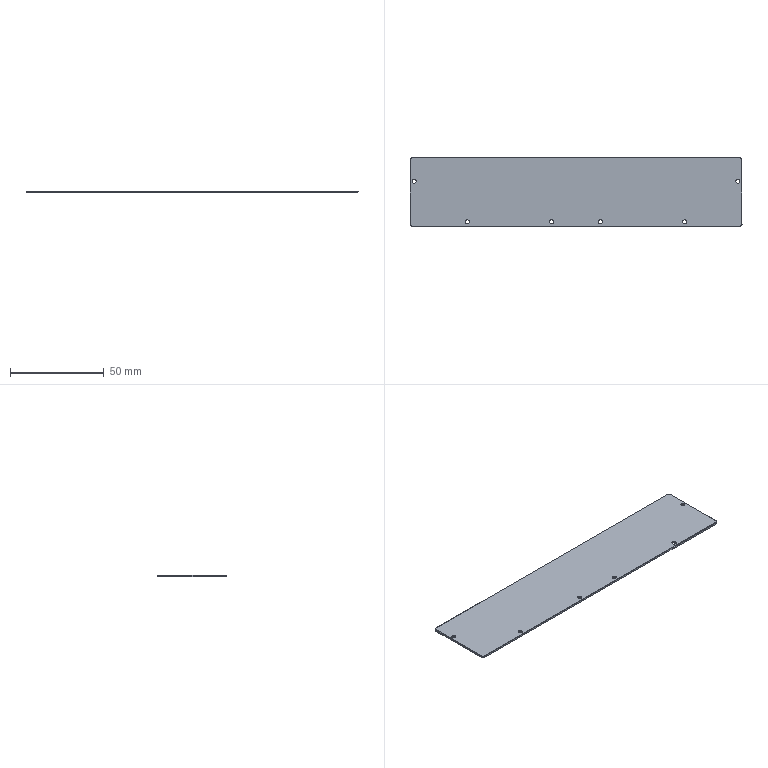Part | SolidWorks | features BaseBody 1 | 1 solid | 42 faces | box 177 x 36.8 x 1 mm | volume 6475 mm3 | cone 16 | cylinder 16 | plane 10 | commonest cylinder face diameters 2.2 x12 2.6 x4
STEP:
#1=CARTESIAN_POINT('',(-59.1,-64.9,0.5));
#2=VERTEX_POINT('',#1);
#3=CARTESIAN_POINT('',(-56.9,-64.9,0.5));
#4=VERTEX_POINT('',#3);
#5=CARTESIAN_POINT('',(-58.,-64.9,0.5));
#6=DIRECTION('',(0.,0.,1.));
#7=DIRECTION('',(0.,-1.,0.));
#8=AXIS2_PLACEMENT_3D('',#5,#6,#7);
#9=CIRCLE('',#8,1.1);
#10=EDGE_CURVE('',#2,#4,#9,.T.);
#11=ORIENTED_EDGE('',*,*,#10,.T.);
#12=CARTESIAN_POINT('',(-56.4,-64.9,0.000000001));
#13=VERTEX_POINT('',#12);
#14=CARTESIAN_POINT('',(-56.9,-64.9,0.5));
#15=DIRECTION('',(0.7071,0.,-0.7071));
#16=VECTOR('',#15,1000.);
#17=LINE('',#14,#16);
#18=EDGE_CURVE('',#4,#13,#17,.T.);
#19=ORIENTED_EDGE('',*,*,#18,.T.);
#20=CARTESIAN_POINT('',(-59.6,-64.9,0.000000001));
#21=VERTEX_POINT('',#20);
#22=CARTESIAN_POINT('',(-58.,-64.9,0.000000001));
#23=DIRECTION('',(0.,0.,-1.));
#24=DIRECTION('',(-1.,0.,0.));
#25=AXIS2_PLACEMENT_3D('',#22,#23,#24);
#26=CIRCLE('',#25,1.6);
#27=EDGE_CURVE('',#13,#21,#26,.T.);
#28=ORIENTED_EDGE('',*,*,#27,.T.);
#29=CARTESIAN_POINT('',(-59.1,-64.9,0.5));
#30=DIRECTION('',(-0.7071,0.,-0.7071));
#31=VECTOR('',#30,1000.);
#32=LINE('',#29,#31);
#33=EDGE_CURVE('',#2,#21,#32,.T.);
#34=ORIENTED_EDGE('',*,*,#33,.F.);
#35=EDGE_LOOP('',(#11,#19,#28,#34));
#36=FACE_OUTER_BOUND('',#35,.T.);
#37=CARTESIAN_POINT('',(-58.,-64.9,0.5));
#38=DIRECTION('',(0.,0.,-1.));
#39=DIRECTION('',(-1.,0.,0.));
#40=AXIS2_PLACEMENT_3D('',#37,#38,#39);
#41=CONICAL_SURFACE('',#40,1.1,0.7854);
#42=ADVANCED_FACE('',(#36),#41,.F.);
#43=CARTESIAN_POINT('',(56.9,-64.9,0.5));
#44=VERTEX_POINT('',#43);
#45=CARTESIAN_POINT('',(59.1,-64.9,0.5));
#46=VERTEX_POINT('',#45);
#47=CARTESIAN_POINT('',(58.,-64.9,0.5));
#48=DIRECTION('',(0.,0.,1.));
#49=DIRECTION('',(0.,-1.,0.));
#50=AXIS2_PLACEMENT_3D('',#47,#48,#49);
#51=CIRCLE('',#50,1.1);
#52=EDGE_CURVE('',#44,#46,#51,.T.);
#53=ORIENTED_EDGE('',*,*,#52,.T.);
#54=CARTESIAN_POINT('',(59.6,-64.9,0.000000001));
#55=VERTEX_POINT('',#54);
#56=CARTESIAN_POINT('',(59.1,-64.9,0.5));
#57=DIRECTION('',(0.7071,0.,-0.7071));
#58=VECTOR('',#57,1000.);
#59=LINE('',#56,#58);
#60=EDGE_CURVE('',#46,#55,#59,.T.);
#61=ORIENTED_EDGE('',*,*,#60,.T.);
#62=CARTESIAN_POINT('',(56.4,-64.9,0.000000001));
#63=VERTEX_POINT('',#62);
#64=CARTESIAN_POINT('',(58.,-64.9,0.000000001));
#65=DIRECTION('',(0.,0.,-1.));
#66=DIRECTION('',(-1.,0.,0.));
#67=AXIS2_PLACEMENT_3D('',#64,#65,#66);
#68=CIRCLE('',#67,1.6);
#69=EDGE_CURVE('',#55,#63,#68,.T.);
#70=ORIENTED_EDGE('',*,*,#69,.T.);
#71=CARTESIAN_POINT('',(56.9,-64.9,0.5));
#72=DIRECTION('',(-0.7071,0.,-0.7071));
#73=VECTOR('',#72,1000.);
#74=LINE('',#71,#73);
#75=EDGE_CURVE('',#44,#63,#74,.T.);
#76=ORIENTED_EDGE('',*,*,#75,.F.);
#77=EDGE_LOOP('',(#53,#61,#70,#76));
#78=FACE_OUTER_BOUND('',#77,.T.);
#79=CARTESIAN_POINT('',(58.,-64.9,0.5));
#80=DIRECTION('',(0.,0.,-1.));
#81=DIRECTION('',(-1.,0.,0.));
#82=AXIS2_PLACEMENT_3D('',#79,#80,#81);
#83=CONICAL_SURFACE('',#82,1.1,0.7854);
#84=ADVANCED_FACE('',(#78),#83,.F.);
#85=CARTESIAN_POINT('',(-87.4,-43.2,0.5));
#86=VERTEX_POINT('',#85);
#87=CARTESIAN_POINT('',(-85.2,-43.2,0.5));
#88=VERTEX_POINT('',#87);
#89=CARTESIAN_POINT('',(-86.3,-43.2,0.5));
#90=DIRECTION('',(0.,0.,1.));
#91=DIRECTION('',(0.,-1.,0.));
#92=AXIS2_PLACEMENT_3D('',#89,#90,#91);
#93=CIRCLE('',#92,1.1);
#94=EDGE_CURVE('',#86,#88,#93,.T.);
#95=ORIENTED_EDGE('',*,*,#94,.T.);
#96=CARTESIAN_POINT('',(-84.7,-43.2,0.000000001));
#97=VERTEX_POINT('',#96);
#98=CARTESIAN_POINT('',(-85.2,-43.2,0.5));
#99=DIRECTION('',(0.7071,0.,-0.7071));
#100=VECTOR('',#99,1000.);
#101=LINE('',#98,#100);
#102=EDGE_CURVE('',#88,#97,#101,.T.);
#103=ORIENTED_EDGE('',*,*,#102,.T.);
#104=CARTESIAN_POINT('',(-87.9,-43.2,0.000000001));
#105=VERTEX_POINT('',#104);
#106=CARTESIAN_POINT('',(-86.3,-43.2,0.000000001));
#107=DIRECTION('',(0.,0.,-1.));
#108=DIRECTION('',(-1.,0.,0.));
#109=AXIS2_PLACEMENT_3D('',#106,#107,#108);
#110=CIRCLE('',#109,1.6);
#111=EDGE_CURVE('',#97,#105,#110,.T.);
#112=ORIENTED_EDGE('',*,*,#111,.T.);
#113=CARTESIAN_POINT('',(-87.4,-43.2,0.5));
#114=DIRECTION('',(-0.7071,0.,-0.7071));
#115=VECTOR('',#114,1000.);
#116=LINE('',#113,#115);
#117=EDGE_CURVE('',#86,#105,#116,.T.);
#118=ORIENTED_EDGE('',*,*,#117,.F.);
#119=EDGE_LOOP('',(#95,#103,#112,#118));
#120=FACE_OUTER_BOUND('',#119,.T.);
#121=CARTESIAN_POINT('',(-86.3,-43.2,0.5));
#122=DIRECTION('',(0.,0.,-1.));
#123=DIRECTION('',(-1.,0.,0.));
#124=AXIS2_PLACEMENT_3D('',#121,#122,#123);
#125=CONICAL_SURFACE('',#124,1.1,0.7854);
#126=ADVANCED_FACE('',(#120),#125,.F.);
#127=CARTESIAN_POINT('',(-14.1,-64.9,0.5));
#128=VERTEX_POINT('',#127);
#129=CARTESIAN_POINT('',(-11.9,-64.9,0.5));
#130=VERTEX_POINT('',#129);
#131=CARTESIAN_POINT('',(-13.,-64.9,0.5));
#132=DIRECTION('',(0.,0.,1.));
#133=DIRECTION('',(0.,-1.,0.));
#134=AXIS2_PLACEMENT_3D('',#131,#132,#133);
#135=CIRCLE('',#134,1.1);
#136=EDGE_CURVE('',#128,#130,#135,.T.);
#137=ORIENTED_EDGE('',*,*,#136,.T.);
#138=CARTESIAN_POINT('',(-11.4,-64.9,0.000000001));
#139=VERTEX_POINT('',#138);
#140=CARTESIAN_POINT('',(-11.9,-64.9,0.5));
#141=DIRECTION('',(0.7071,0.,-0.7071));
#142=VECTOR('',#141,1000.);
#143=LINE('',#140,#142);
#144=EDGE_CURVE('',#130,#139,#143,.T.);
#145=ORIENTED_EDGE('',*,*,#144,.T.);
#146=CARTESIAN_POINT('',(-14.6,-64.9,0.000000001));
#147=VERTEX_POINT('',#146);
#148=CARTESIAN_POINT('',(-13.,-64.9,0.000000001));
#149=DIRECTION('',(0.,0.,-1.));
#150=DIRECTION('',(-1.,0.,0.));
#151=AXIS2_PLACEMENT_3D('',#148,#149,#150);
#152=CIRCLE('',#151,1.6);
#153=EDGE_CURVE('',#139,#147,#152,.T.);
#154=ORIENTED_EDGE('',*,*,#153,.T.);
#155=CARTESIAN_POINT('',(-14.1,-64.9,0.5));
#156=DIRECTION('',(-0.7071,0.,-0.7071));
#157=VECTOR('',#156,1000.);
#158=LINE('',#155,#157);
#159=EDGE_CURVE('',#128,#147,#158,.T.);
#160=ORIENTED_EDGE('',*,*,#159,.F.);
#161=EDGE_LOOP('',(#137,#145,#154,#160));
#162=FACE_OUTER_BOUND('',#161,.T.);
#163=CARTESIAN_POINT('',(-13.,-64.9,0.5));
#164=DIRECTION('',(0.,0.,-1.));
#165=DIRECTION('',(-1.,0.,0.));
#166=AXIS2_PLACEMENT_3D('',#163,#164,#165);
#167=CONICAL_SURFACE('',#166,1.1,0.7854);
#168=ADVANCED_FACE('',(#162),#167,.F.);
#169=CARTESIAN_POINT('',(11.9,-64.9,0.5));
#170=VERTEX_POINT('',#169);
#171=CARTESIAN_POINT('',(14.1,-64.9,0.5));
#172=VERTEX_POINT('',#171);
#173=CARTESIAN_POINT('',(13.,-64.9,0.5));
#174=DIRECTION('',(0.,0.,1.));
#175=DIRECTION('',(0.,-1.,0.));
#176=AXIS2_PLACEMENT_3D('',#173,#174,#175);
#177=CIRCLE('',#176,1.1);
#178=EDGE_CURVE('',#170,#172,#177,.T.);
#179=ORIENTED_EDGE('',*,*,#178,.T.);
#180=CARTESIAN_POINT('',(14.6,-64.9,0.000000001));
#181=VERTEX_POINT('',#180);
#182=CARTESIAN_POINT('',(14.1,-64.9,0.5));
#183=DIRECTION('',(0.7071,0.,-0.7071));
#184=VECTOR('',#183,1000.);
#185=LINE('',#182,#184);
#186=EDGE_CURVE('',#172,#181,#185,.T.);
#187=ORIENTED_EDGE('',*,*,#186,.T.);
#188=CARTESIAN_POINT('',(11.4,-64.9,0.000000001));
#189=VERTEX_POINT('',#188);
#190=CARTESIAN_POINT('',(13.,-64.9,0.000000001));
#191=DIRECTION('',(0.,0.,-1.));
#192=DIRECTION('',(-1.,0.,0.));
#193=AXIS2_PLACEMENT_3D('',#190,#191,#192);
#194=CIRCLE('',#193,1.6);
#195=EDGE_CURVE('',#181,#189,#194,.T.);
#196=ORIENTED_EDGE('',*,*,#195,.T.);
#197=CARTESIAN_POINT('',(11.9,-64.9,0.5));
#198=DIRECTION('',(-0.7071,0.,-0.7071));
#199=VECTOR('',#198,1000.);
#200=LINE('',#197,#199);
#201=EDGE_CURVE('',#170,#189,#200,.T.);
#202=ORIENTED_EDGE('',*,*,#201,.F.);
#203=EDGE_LOOP('',(#179,#187,#196,#202));
#204=FACE_OUTER_BOUND('',#203,.T.);
#205=CARTESIAN_POINT('',(13.,-64.9,0.5));
#206=DIRECTION('',(0.,0.,-1.));
#207=DIRECTION('',(-1.,0.,0.));
#208=AXIS2_PLACEMENT_3D('',#205,#206,#207);
#209=CONICAL_SURFACE('',#208,1.1,0.7854);
#210=ADVANCED_FACE('',(#204),#209,.F.);
#211=CARTESIAN_POINT('',(85.2,-43.2,0.5));
#212=VERTEX_POINT('',#211);
#213=CARTESIAN_POINT('',(87.4,-43.2,0.5));
#214=VERTEX_POINT('',#213);
#215=CARTESIAN_POINT('',(86.3,-43.2,0.5));
#216=DIRECTION('',(0.,0.,1.));
#217=DIRECTION('',(0.,-1.,0.));
#218=AXIS2_PLACEMENT_3D('',#215,#216,#217);
#219=CIRCLE('',#218,1.1);
#220=EDGE_CURVE('',#212,#214,#219,.T.);
#221=ORIENTED_EDGE('',*,*,#220,.T.);
#222=CARTESIAN_POINT('',(87.9,-43.2,0.000000001));
#223=VERTEX_POINT('',#222);
#224=CARTESIAN_POINT('',(87.4,-43.2,0.5));
#225=DIRECTION('',(0.7071,0.,-0.7071));
#226=VECTOR('',#225,1000.);
#227=LINE('',#224,#226);
#228=EDGE_CURVE('',#214,#223,#227,.T.);
#229=ORIENTED_EDGE('',*,*,#228,.T.);
#230=CARTESIAN_POINT('',(84.7,-43.2,0.000000001));
#231=VERTEX_POINT('',#230);
#232=CARTESIAN_POINT('',(86.3,-43.2,0.000000001));
#233=DIRECTION('',(0.,0.,-1.));
#234=DIRECTION('',(-1.,0.,0.));
#235=AXIS2_PLACEMENT_3D('',#232,#233,#234);
#236=CIRCLE('',#235,1.6);
#237=EDGE_CURVE('',#223,#231,#236,.T.);
#238=ORIENTED_EDGE('',*,*,#237,.T.);
#239=CARTESIAN_POINT('',(85.2,-43.2,0.5));
#240=DIRECTION('',(-0.7071,0.,-0.7071));
#241=VECTOR('',#240,1000.);
#242=LINE('',#239,#241);
#243=EDGE_CURVE('',#212,#231,#242,.T.);
#244=ORIENTED_EDGE('',*,*,#243,.F.);
#245=EDGE_LOOP('',(#221,#229,#238,#244));
#246=FACE_OUTER_BOUND('',#245,.T.);
#247=CARTESIAN_POINT('',(86.3,-43.2,0.5));
#248=DIRECTION('',(0.,0.,-1.));
#249=DIRECTION('',(-1.,0.,0.));
#250=AXIS2_PLACEMENT_3D('',#247,#248,#249);
#251=CONICAL_SURFACE('',#250,1.1,0.7854);
#252=ADVANCED_FACE('',(#246),#251,.F.);
#253=CARTESIAN_POINT('',(-59.1,-64.9,1.));
#254=VERTEX_POINT('',#253);
#255=CARTESIAN_POINT('',(-56.9,-64.9,1.));
#256=VERTEX_POINT('',#255);
#257=CARTESIAN_POINT('',(-58.,-64.9,1.));
#258=DIRECTION('',(0.,0.,1.));
#259=DIRECTION('',(-1.,0.,0.));
#260=AXIS2_PLACEMENT_3D('',#257,#258,#259);
#261=CIRCLE('',#260,1.1);
#262=EDGE_CURVE('',#254,#256,#261,.T.);
#263=ORIENTED_EDGE('',*,*,#262,.T.);
#264=CARTESIAN_POINT('',(-56.9,-64.9,1.));
#265=DIRECTION('',(0.,0.,-1.));
#266=VECTOR('',#265,1000.);
#267=LINE('',#264,#266);
#268=EDGE_CURVE('',#256,#4,#267,.T.);
#269=ORIENTED_EDGE('',*,*,#268,.T.);
#270=ORIENTED_EDGE('',*,*,#10,.F.);
#271=CARTESIAN_POINT('',(-59.1,-64.9,1.));
#272=DIRECTION('',(0.,0.,-1.));
#273=VECTOR('',#272,1000.);
#274=LINE('',#271,#273);
#275=EDGE_CURVE('',#254,#2,#274,.T.);
#276=ORIENTED_EDGE('',*,*,#275,.F.);
#277=EDGE_LOOP('',(#263,#269,#270,#276));
#278=FACE_OUTER_BOUND('',#277,.T.);
#279=CARTESIAN_POINT('',(-58.,-64.9,1.));
#280=DIRECTION('',(0.,0.,-1.));
#281=DIRECTION('',(-1.,0.,0.));
#282=AXIS2_PLACEMENT_3D('',#279,#280,#281);
#283=CYLINDRICAL_SURFACE('',#282,1.1);
#284=ADVANCED_FACE('',(#278),#283,.F.);
#285=CARTESIAN_POINT('',(56.9,-64.9,1.));
#286=VERTEX_POINT('',#285);
#287=CARTESIAN_POINT('',(59.1,-64.9,1.));
#288=VERTEX_POINT('',#287);
#289=CARTESIAN_POINT('',(58.,-64.9,1.));
#290=DIRECTION('',(0.,0.,1.));
#291=DIRECTION('',(-1.,0.,0.));
#292=AXIS2_PLACEMENT_3D('',#289,#290,#291);
#293=CIRCLE('',#292,1.1);
#294=EDGE_CURVE('',#286,#288,#293,.T.);
#295=ORIENTED_EDGE('',*,*,#294,.T.);
#296=CARTESIAN_POINT('',(59.1,-64.9,1.));
#297=DIRECTION('',(0.,0.,-1.));
#298=VECTOR('',#297,1000.);
#299=LINE('',#296,#298);
#300=EDGE_CURVE('',#288,#46,#299,.T.);
#301=ORIENTED_EDGE('',*,*,#300,.T.);
#302=ORIENTED_EDGE('',*,*,#52,.F.);
#303=CARTESIAN_POINT('',(56.9,-64.9,1.));
#304=DIRECTION('',(0.,0.,-1.));
#305=VECTOR('',#304,1000.);
#306=LINE('',#303,#305);
#307=EDGE_CURVE('',#286,#44,#306,.T.);
#308=ORIENTED_EDGE('',*,*,#307,.F.);
#309=EDGE_LOOP('',(#295,#301,#302,#308));
#310=FACE_OUTER_BOUND('',#309,.T.);
#311=CARTESIAN_POINT('',(58.,-64.9,1.));
#312=DIRECTION('',(0.,0.,-1.));
#313=DIRECTION('',(-1.,0.,0.));
#314=AXIS2_PLACEMENT_3D('',#311,#312,#313);
#315=CYLINDRICAL_SURFACE('',#314,1.1);
#316=ADVANCED_FACE('',(#310),#315,.F.);
#317=CARTESIAN_POINT('',(-87.4,-43.2,1.));
#318=VERTEX_POINT('',#317);
#319=CARTESIAN_POINT('',(-85.2,-43.2,1.));
#320=VERTEX_POINT('',#319);
#321=CARTESIAN_POINT('',(-86.3,-43.2,1.));
#322=DIRECTION('',(0.,0.,1.));
#323=DIRECTION('',(-1.,0.,0.));
#324=AXIS2_PLACEMENT_3D('',#321,#322,#323);
#325=CIRCLE('',#324,1.1);
#326=EDGE_CURVE('',#318,#320,#325,.T.);
#327=ORIENTED_EDGE('',*,*,#326,.T.);
#328=CARTESIAN_POINT('',(-85.2,-43.2,1.));
#329=DIRECTION('',(0.,0.,-1.));
#330=VECTOR('',#329,1000.);
#331=LINE('',#328,#330);
#332=EDGE_CURVE('',#320,#88,#331,.T.);
#333=ORIENTED_EDGE('',*,*,#332,.T.);
#334=ORIENTED_EDGE('',*,*,#94,.F.);
#335=CARTESIAN_POINT('',(-87.4,-43.2,1.));
#336=DIRECTION('',(0.,0.,-1.));
#337=VECTOR('',#336,1000.);
#338=LINE('',#335,#337);
#339=EDGE_CURVE('',#318,#86,#338,.T.);
#340=ORIENTED_EDGE('',*,*,#339,.F.);
#341=EDGE_LOOP('',(#327,#333,#334,#340));
#342=FACE_OUTER_BOUND('',#341,.T.);
#343=CARTESIAN_POINT('',(-86.3,-43.2,1.));
#344=DIRECTION('',(0.,0.,-1.));
#345=DIRECTION('',(-1.,0.,0.));
#346=AXIS2_PLACEMENT_3D('',#343,#344,#345);
#347=CYLINDRICAL_SURFACE('',#346,1.1);
#348=ADVANCED_FACE('',(#342),#347,.F.);
#349=CARTESIAN_POINT('',(-14.1,-64.9,1.));
#350=VERTEX_POINT('',#349);
#351=CARTESIAN_POINT('',(-11.9,-64.9,1.));
#352=VERTEX_POINT('',#351);
#353=CARTESIAN_POINT('',(-13.,-64.9,1.));
#354=DIRECTION('',(0.,0.,1.));
#355=DIRECTION('',(-1.,0.,0.));
#356=AXIS2_PLACEMENT_3D('',#353,#354,#355);
#357=CIRCLE('',#356,1.1);
#358=EDGE_CURVE('',#350,#352,#357,.T.);
#359=ORIENTED_EDGE('',*,*,#358,.T.);
#360=CARTESIAN_POINT('',(-11.9,-64.9,1.));
#361=DIRECTION('',(0.,0.,-1.));
#362=VECTOR('',#361,1000.);
#363=LINE('',#360,#362);
#364=EDGE_CURVE('',#352,#130,#363,.T.);
#365=ORIENTED_EDGE('',*,*,#364,.T.);
#366=ORIENTED_EDGE('',*,*,#136,.F.);
#367=CARTESIAN_POINT('',(-14.1,-64.9,1.));
#368=DIRECTION('',(0.,0.,-1.));
#369=VECTOR('',#368,1000.);
#370=LINE('',#367,#369);
#371=EDGE_CURVE('',#350,#128,#370,.T.);
#372=ORIENTED_EDGE('',*,*,#371,.F.);
#373=EDGE_LOOP('',(#359,#365,#366,#372));
#374=FACE_OUTER_BOUND('',#373,.T.);
#375=CARTESIAN_POINT('',(-13.,-64.9,1.));
#376=DIRECTION('',(0.,0.,-1.));
#377=DIRECTION('',(-1.,0.,0.));
#378=AXIS2_PLACEMENT_3D('',#375,#376,#377);
#379=CYLINDRICAL_SURFACE('',#378,1.1);
#380=ADVANCED_FACE('',(#374),#379,.F.);
#381=CARTESIAN_POINT('',(11.9,-64.9,1.));
#382=VERTEX_POINT('',#381);
#383=CARTESIAN_POINT('',(14.1,-64.9,1.));
#384=VERTEX_POINT('',#383);
#385=CARTESIAN_POINT('',(13.,-64.9,1.));
#386=DIRECTION('',(0.,0.,1.));
#387=DIRECTION('',(-1.,0.,0.));
#388=AXIS2_PLACEMENT_3D('',#385,#386,#387);
#389=CIRCLE('',#388,1.1);
#390=EDGE_CURVE('',#382,#384,#389,.T.);
#391=ORIENTED_EDGE('',*,*,#390,.T.);
#392=CARTESIAN_POINT('',(14.1,-64.9,1.));
#393=DIRECTION('',(0.,0.,-1.));
#394=VECTOR('',#393,1000.);
#395=LINE('',#392,#394);
#396=EDGE_CURVE('',#384,#172,#395,.T.);
#397=ORIENTED_EDGE('',*,*,#396,.T.);
#398=ORIENTED_EDGE('',*,*,#178,.F.);
#399=CARTESIAN_POINT('',(11.9,-64.9,1.));
#400=DIRECTION('',(0.,0.,-1.));
#401=VECTOR('',#400,1000.);
#402=LINE('',#399,#401);
#403=EDGE_CURVE('',#382,#170,#402,.T.);
#404=ORIENTED_EDGE('',*,*,#403,.F.);
#405=EDGE_LOOP('',(#391,#397,#398,#404));
#406=FACE_OUTER_BOUND('',#405,.T.);
#407=CARTESIAN_POINT('',(13.,-64.9,1.));
#408=DIRECTION('',(0.,0.,-1.));
#409=DIRECTION('',(-1.,0.,0.));
#410=AXIS2_PLACEMENT_3D('',#407,#408,#409);
#411=CYLINDRICAL_SURFACE('',#410,1.1);
#412=ADVANCED_FACE('',(#406),#411,.F.);
#413=CARTESIAN_POINT('',(85.2,-43.2,1.));
#414=VERTEX_POINT('',#413);
#415=CARTESIAN_POINT('',(87.4,-43.2,1.));
#416=VERTEX_POINT('',#415);
#417=CARTESIAN_POINT('',(86.3,-43.2,1.));
#418=DIRECTION('',(0.,0.,1.));
#419=DIRECTION('',(-1.,0.,0.));
#420=AXIS2_PLACEMENT_3D('',#417,#418,#419);
#421=CIRCLE('',#420,1.1);
#422=EDGE_CURVE('',#414,#416,#421,.T.);
#423=ORIENTED_EDGE('',*,*,#422,.T.);
#424=CARTESIAN_POINT('',(87.4,-43.2,1.));
#425=DIRECTION('',(0.,0.,-1.));
#426=VECTOR('',#425,1000.);
#427=LINE('',#424,#426);
#428=EDGE_CURVE('',#416,#214,#427,.T.);
#429=ORIENTED_EDGE('',*,*,#428,.T.);
#430=ORIENTED_EDGE('',*,*,#220,.F.);
#431=CARTESIAN_POINT('',(85.2,-43.2,1.));
#432=DIRECTION('',(0.,0.,-1.));
#433=VECTOR('',#432,1000.);
#434=LINE('',#431,#433);
#435=EDGE_CURVE('',#414,#212,#434,.T.);
#436=ORIENTED_EDGE('',*,*,#435,.F.);
#437=EDGE_LOOP('',(#423,#429,#430,#436));
#438=FACE_OUTER_BOUND('',#437,.T.);
#439=CARTESIAN_POINT('',(86.3,-43.2,1.));
#440=DIRECTION('',(0.,0.,-1.));
#441=DIRECTION('',(-1.,0.,0.));
#442=AXIS2_PLACEMENT_3D('',#439,#440,#441);
#443=CYLINDRICAL_SURFACE('',#442,1.1);
#444=ADVANCED_FACE('',(#438),#443,.F.);
#445=CARTESIAN_POINT('',(-58.,-64.9,0.000000001));
#446=DIRECTION('',(0.,0.,-1.));
#447=DIRECTION('',(-1.,0.,0.));
#448=AXIS2_PLACEMENT_3D('',#445,#446,#447);
#449=CIRCLE('',#448,1.6);
#450=EDGE_CURVE('',#21,#13,#449,.T.);
#451=ORIENTED_EDGE('',*,*,#450,.F.);
#452=ORIENTED_EDGE('',*,*,#27,.F.);
#453=EDGE_LOOP('',(#451,#452));
#454=FACE_BOUND('',#453,.T.);
#455=CARTESIAN_POINT('',(58.,-64.9,0.000000001));
#456=DIRECTION('',(0.,0.,-1.));
#457=DIRECTION('',(-1.,0.,0.));
#458=AXIS2_PLACEMENT_3D('',#455,#456,#457);
#459=CIRCLE('',#458,1.6);
#460=EDGE_CURVE('',#63,#55,#459,.T.);
#461=ORIENTED_EDGE('',*,*,#460,.F.);
#462=ORIENTED_EDGE('',*,*,#69,.F.);
#463=EDGE_LOOP('',(#461,#462));
#464=FACE_BOUND('',#463,.T.);
#465=CARTESIAN_POINT('',(-86.3,-43.2,0.000000001));
#466=DIRECTION('',(0.,0.,-1.));
#467=DIRECTION('',(-1.,0.,0.));
#468=AXIS2_PLACEMENT_3D('',#465,#466,#467);
#469=CIRCLE('',#468,1.6);
#470=EDGE_CURVE('',#105,#97,#469,.T.);
#471=ORIENTED_EDGE('',*,*,#470,.F.);
#472=ORIENTED_EDGE('',*,*,#111,.F.);
#473=EDGE_LOOP('',(#471,#472));
#474=FACE_BOUND('',#473,.T.);
#475=CARTESIAN_POINT('',(-13.,-64.9,0.000000001));
#476=DIRECTION('',(0.,0.,-1.));
#477=DIRECTION('',(-1.,0.,0.));
#478=AXIS2_PLACEMENT_3D('',#475,#476,#477);
#479=CIRCLE('',#478,1.6);
#480=EDGE_CURVE('',#147,#139,#479,.T.);
#481=ORIENTED_EDGE('',*,*,#480,.F.);
#482=ORIENTED_EDGE('',*,*,#153,.F.);
#483=EDGE_LOOP('',(#481,#482));
#484=FACE_BOUND('',#483,.T.);
#485=CARTESIAN_POINT('',(13.,-64.9,0.000000001));
#486=DIRECTION('',(0.,0.,-1.));
#487=DIRECTION('',(-1.,0.,0.));
#488=AXIS2_PLACEMENT_3D('',#485,#486,#487);
#489=CIRCLE('',#488,1.6);
#490=EDGE_CURVE('',#189,#181,#489,.T.);
#491=ORIENTED_EDGE('',*,*,#490,.F.);
#492=ORIENTED_EDGE('',*,*,#195,.F.);
#493=EDGE_LOOP('',(#491,#492));
#494=FACE_BOUND('',#493,.T.);
#495=CARTESIAN_POINT('',(86.3,-43.2,0.000000001));
#496=DIRECTION('',(0.,0.,-1.));
#497=DIRECTION('',(-1.,0.,0.));
#498=AXIS2_PLACEMENT_3D('',#495,#496,#497);
#499=CIRCLE('',#498,1.6);
#500=EDGE_CURVE('',#231,#223,#499,.T.);
#501=ORIENTED_EDGE('',*,*,#500,.F.);
#502=ORIENTED_EDGE('',*,*,#237,.F.);
#503=EDGE_LOOP('',(#501,#502));
#504=FACE_BOUND('',#503,.T.);
#505=CARTESIAN_POINT('',(88.5,-31.9,0.));
#506=VERTEX_POINT('',#505);
#507=CARTESIAN_POINT('',(87.2,-30.6,0.));
#508=VERTEX_POINT('',#507);
#509=CARTESIAN_POINT('',(87.2,-31.9,0.));
#510=DIRECTION('',(0.,0.,1.));
#511=DIRECTION('',(-1.,0.,0.));
#512=AXIS2_PLACEMENT_3D('',#509,#510,#511);
#513=CIRCLE('',#512,1.3);
#514=EDGE_CURVE('',#506,#508,#513,.T.);
#515=ORIENTED_EDGE('',*,*,#514,.F.);
#516=CARTESIAN_POINT('',(88.5,-66.1,0.));
#517=VERTEX_POINT('',#516);
#518=CARTESIAN_POINT('',(88.5,-49.,0.));
#519=DIRECTION('',(0.,1.,0.));
#520=VECTOR('',#519,1000.);
#521=LINE('',#518,#520);
#522=EDGE_CURVE('',#517,#506,#521,.T.);
#523=ORIENTED_EDGE('',*,*,#522,.F.);
#524=CARTESIAN_POINT('',(87.2,-67.4,0.));
#525=VERTEX_POINT('',#524);
#526=CARTESIAN_POINT('',(87.2,-66.1,0.));
#527=DIRECTION('',(0.,0.,1.));
#528=DIRECTION('',(-1.,0.,0.));
#529=AXIS2_PLACEMENT_3D('',#526,#527,#528);
#530=CIRCLE('',#529,1.3);
#531=EDGE_CURVE('',#525,#517,#530,.T.);
#532=ORIENTED_EDGE('',*,*,#531,.F.);
#533=CARTESIAN_POINT('',(-87.2,-67.4,0.));
#534=VERTEX_POINT('',#533);
#535=CARTESIAN_POINT('',(0.,-67.4,0.));
#536=DIRECTION('',(1.,0.,0.));
#537=VECTOR('',#536,1000.);
#538=LINE('',#535,#537);
#539=EDGE_CURVE('',#534,#525,#538,.T.);
#540=ORIENTED_EDGE('',*,*,#539,.F.);
#541=CARTESIAN_POINT('',(-88.5,-66.1,0.));
#542=VERTEX_POINT('',#541);
#543=CARTESIAN_POINT('',(-87.2,-66.1,0.));
#544=DIRECTION('',(0.,0.,1.));
#545=DIRECTION('',(-1.,0.,0.));
#546=AXIS2_PLACEMENT_3D('',#543,#544,#545);
#547=CIRCLE('',#546,1.3);
#548=EDGE_CURVE('',#542,#534,#547,.T.);
#549=ORIENTED_EDGE('',*,*,#548,.F.);
#550=CARTESIAN_POINT('',(-88.5,-31.9,0.));
#551=VERTEX_POINT('',#550);
#552=CARTESIAN_POINT('',(-88.5,-49.,0.));
#553=DIRECTION('',(0.,-1.,0.));
#554=VECTOR('',#553,1000.);
#555=LINE('',#552,#554);
#556=EDGE_CURVE('',#551,#542,#555,.T.);
#557=ORIENTED_EDGE('',*,*,#556,.F.);
#558=CARTESIAN_POINT('',(-87.2,-30.6,0.));
#559=VERTEX_POINT('',#558);
#560=CARTESIAN_POINT('',(-87.2,-31.9,0.));
#561=DIRECTION('',(0.,0.,1.));
#562=DIRECTION('',(-1.,0.,0.));
#563=AXIS2_PLACEMENT_3D('',#560,#561,#562);
#564=CIRCLE('',#563,1.3);
#565=EDGE_CURVE('',#559,#551,#564,.T.);
#566=ORIENTED_EDGE('',*,*,#565,.F.);
#567=CARTESIAN_POINT('',(0.,-30.6,0.));
#568=DIRECTION('',(-1.,0.,0.));
#569=VECTOR('',#568,1000.);
#570=LINE('',#567,#569);
#571=EDGE_CURVE('',#508,#559,#570,.T.);
#572=ORIENTED_EDGE('',*,*,#571,.F.);
#573=EDGE_LOOP('',(#515,#523,#532,#540,#549,#557,#566,#572));
#574=FACE_OUTER_BOUND('',#573,.T.);
#575=CARTESIAN_POINT('',(92.04,-68.136,0.));
#576=DIRECTION('',(0.,0.,1.));
#577=DIRECTION('',(0.,1.,0.));
#578=AXIS2_PLACEMENT_3D('',#575,#576,#577);
#579=PLANE('',#578);
#580=ADVANCED_FACE('',(#454,#464,#474,#484,#494,#504,#574),#579,.F.);
#581=ORIENTED_EDGE('',*,*,#18,.F.);
#582=CARTESIAN_POINT('',(-58.,-64.9,0.5));
#583=DIRECTION('',(0.,0.,1.));
#584=DIRECTION('',(0.,-1.,0.));
#585=AXIS2_PLACEMENT_3D('',#582,#583,#584);
#586=CIRCLE('',#585,1.1);
#587=EDGE_CURVE('',#4,#2,#586,.T.);
#588=ORIENTED_EDGE('',*,*,#587,.T.);
#589=ORIENTED_EDGE('',*,*,#33,.T.);
#590=ORIENTED_EDGE('',*,*,#450,.T.);
#591=EDGE_LOOP('',(#581,#588,#589,#590));
#592=FACE_OUTER_BOUND('',#591,.T.);
#593=CARTESIAN_POINT('',(-58.,-64.9,0.5));
#594=DIRECTION('',(0.,0.,-1.));
#595=DIRECTION('',(-1.,0.,0.));
#596=AXIS2_PLACEMENT_3D('',#593,#594,#595);
#597=CONICAL_SURFACE('',#596,1.1,0.7854);
#598=ADVANCED_FACE('',(#592),#597,.F.);
#599=ORIENTED_EDGE('',*,*,#60,.F.);
#600=CARTESIAN_POINT('',(58.,-64.9,0.5));
#601=DIRECTION('',(0.,0.,1.));
#602=DIRECTION('',(0.,-1.,0.));
#603=AXIS2_PLACEMENT_3D('',#600,#601,#602);
#604=CIRCLE('',#603,1.1);
#605=EDGE_CURVE('',#46,#44,#604,.T.);
#606=ORIENTED_EDGE('',*,*,#605,.T.);
#607=ORIENTED_EDGE('',*,*,#75,.T.);
#608=ORIENTED_EDGE('',*,*,#460,.T.);
#609=EDGE_LOOP('',(#599,#606,#607,#608));
#610=FACE_OUTER_BOUND('',#609,.T.);
#611=CARTESIAN_POINT('',(58.,-64.9,0.5));
#612=DIRECTION('',(0.,0.,-1.));
#613=DIRECTION('',(-1.,0.,0.));
#614=AXIS2_PLACEMENT_3D('',#611,#612,#613);
#615=CONICAL_SURFACE('',#614,1.1,0.7854);
#616=ADVANCED_FACE('',(#610),#615,.F.);
#617=ORIENTED_EDGE('',*,*,#102,.F.);
#618=CARTESIAN_POINT('',(-86.3,-43.2,0.5));
#619=DIRECTION('',(0.,0.,1.));
#620=DIRECTION('',(0.,-1.,0.));
#621=AXIS2_PLACEMENT_3D('',#618,#619,#620);
#622=CIRCLE('',#621,1.1);
#623=EDGE_CURVE('',#88,#86,#622,.T.);
#624=ORIENTED_EDGE('',*,*,#623,.T.);
#625=ORIENTED_EDGE('',*,*,#117,.T.);
#626=ORIENTED_EDGE('',*,*,#470,.T.);
#627=EDGE_LOOP('',(#617,#624,#625,#626));
#628=FACE_OUTER_BOUND('',#627,.T.);
#629=CARTESIAN_POINT('',(-86.3,-43.2,0.5));
#630=DIRECTION('',(0.,0.,-1.));
#631=DIRECTION('',(-1.,0.,0.));
#632=AXIS2_PLACEMENT_3D('',#629,#630,#631);
#633=CONICAL_SURFACE('',#632,1.1,0.7854);
#634=ADVANCED_FACE('',(#628),#633,.F.);
#635=ORIENTED_EDGE('',*,*,#144,.F.);
#636=CARTESIAN_POINT('',(-13.,-64.9,0.5));
#637=DIRECTION('',(0.,0.,1.));
#638=DIRECTION('',(0.,-1.,0.));
#639=AXIS2_PLACEMENT_3D('',#636,#637,#638);
#640=CIRCLE('',#639,1.1);
#641=EDGE_CURVE('',#130,#128,#640,.T.);
#642=ORIENTED_EDGE('',*,*,#641,.T.);
#643=ORIENTED_EDGE('',*,*,#159,.T.);
#644=ORIENTED_EDGE('',*,*,#480,.T.);
#645=EDGE_LOOP('',(#635,#642,#643,#644));
#646=FACE_OUTER_BOUND('',#645,.T.);
#647=CARTESIAN_POINT('',(-13.,-64.9,0.5));
#648=DIRECTION('',(0.,0.,-1.));
#649=DIRECTION('',(-1.,0.,0.));
#650=AXIS2_PLACEMENT_3D('',#647,#648,#649);
#651=CONICAL_SURFACE('',#650,1.1,0.7854);
#652=ADVANCED_FACE('',(#646),#651,.F.);
#653=ORIENTED_EDGE('',*,*,#186,.F.);
#654=CARTESIAN_POINT('',(13.,-64.9,0.5));
#655=DIRECTION('',(0.,0.,1.));
#656=DIRECTION('',(0.,-1.,0.));
#657=AXIS2_PLACEMENT_3D('',#654,#655,#656);
#658=CIRCLE('',#657,1.1);
#659=EDGE_CURVE('',#172,#170,#658,.T.);
#660=ORIENTED_EDGE('',*,*,#659,.T.);
#661=ORIENTED_EDGE('',*,*,#201,.T.);
#662=ORIENTED_EDGE('',*,*,#490,.T.);
#663=EDGE_LOOP('',(#653,#660,#661,#662));
#664=FACE_OUTER_BOUND('',#663,.T.);
#665=CARTESIAN_POINT('',(13.,-64.9,0.5));
#666=DIRECTION('',(0.,0.,-1.));
#667=DIRECTION('',(-1.,0.,0.));
#668=AXIS2_PLACEMENT_3D('',#665,#666,#667);
#669=CONICAL_SURFACE('',#668,1.1,0.7854);
#670=ADVANCED_FACE('',(#664),#669,.F.);
#671=ORIENTED_EDGE('',*,*,#228,.F.);
#672=CARTESIAN_POINT('',(86.3,-43.2,0.5));
#673=DIRECTION('',(0.,0.,1.));
#674=DIRECTION('',(0.,-1.,0.));
#675=AXIS2_PLACEMENT_3D('',#672,#673,#674);
#676=CIRCLE('',#675,1.1);
#677=EDGE_CURVE('',#214,#212,#676,.T.);
#678=ORIENTED_EDGE('',*,*,#677,.T.);
#679=ORIENTED_EDGE('',*,*,#243,.T.);
#680=ORIENTED_EDGE('',*,*,#500,.T.);
#681=EDGE_LOOP('',(#671,#678,#679,#680));
#682=FACE_OUTER_BOUND('',#681,.T.);
#683=CARTESIAN_POINT('',(86.3,-43.2,0.5));
#684=DIRECTION('',(0.,0.,-1.));
#685=DIRECTION('',(-1.,0.,0.));
#686=AXIS2_PLACEMENT_3D('',#683,#684,#685);
#687=CONICAL_SURFACE('',#686,1.1,0.7854);
#688=ADVANCED_FACE('',(#682),#687,.F.);
#689=ORIENTED_EDGE('',*,*,#571,.T.);
#690=CARTESIAN_POINT('',(-87.2,-30.6,0.8));
#691=VERTEX_POINT('',#690);
#692=CARTESIAN_POINT('',(-87.2,-30.6,0.4));
#693=DIRECTION('',(0.,0.,1.));
#694=VECTOR('',#693,1000.);
#695=LINE('',#692,#694);
#696=EDGE_CURVE('',#559,#691,#695,.T.);
#697=ORIENTED_EDGE('',*,*,#696,.T.);
#698=CARTESIAN_POINT('',(87.2,-30.6,0.8));
#699=VERTEX_POINT('',#698);
#700=CARTESIAN_POINT('',(0.,-30.6,0.8));
#701=DIRECTION('',(1.,0.,0.));
#702=VECTOR('',#701,1000.);
#703=LINE('',#700,#702);
#704=EDGE_CURVE('',#691,#699,#703,.T.);
#705=ORIENTED_EDGE('',*,*,#704,.T.);
#706=CARTESIAN_POINT('',(87.2,-30.6,0.4));
#707=DIRECTION('',(0.,0.,-1.));
#708=VECTOR('',#707,1000.);
#709=LINE('',#706,#708);
#710=EDGE_CURVE('',#699,#508,#709,.T.);
#711=ORIENTED_EDGE('',*,*,#710,.T.);
#712=EDGE_LOOP('',(#689,#697,#705,#711));
#713=FACE_OUTER_BOUND('',#712,.T.);
#714=CARTESIAN_POINT('',(90.688,-30.6,-0.2629));
#715=DIRECTION('',(0.,1.,0.));
#716=DIRECTION('',(-1.,0.,0.));
#717=AXIS2_PLACEMENT_3D('',#714,#715,#716);
#718=PLANE('',#717);
#719=ADVANCED_FACE('',(#713),#718,.T.);
#720=ORIENTED_EDGE('',*,*,#514,.T.);
#721=ORIENTED_EDGE('',*,*,#710,.F.);
#722=CARTESIAN_POINT('',(88.5,-31.9,0.8));
#723=VERTEX_POINT('',#722);
#724=CARTESIAN_POINT('',(87.2,-31.9,0.8));
#725=DIRECTION('',(0.,0.,1.));
#726=DIRECTION('',(0.,1.,0.));
#727=AXIS2_PLACEMENT_3D('',#724,#725,#726);
#728=CIRCLE('',#727,1.3);
#729=EDGE_CURVE('',#723,#699,#728,.T.);
#730=ORIENTED_EDGE('',*,*,#729,.F.);
#731=CARTESIAN_POINT('',(88.5,-31.9,0.4));
#732=DIRECTION('',(0.,0.,1.));
#733=VECTOR('',#732,1000.);
#734=LINE('',#731,#733);
#735=EDGE_CURVE('',#506,#723,#734,.T.);
#736=ORIENTED_EDGE('',*,*,#735,.F.);
#737=EDGE_LOOP('',(#720,#721,#730,#736));
#738=FACE_OUTER_BOUND('',#737,.T.);
#739=CARTESIAN_POINT('',(87.2,-31.9,0.8));
#740=DIRECTION('',(0.,0.,-1.));
#741=DIRECTION('',(-1.,0.,0.));
#742=AXIS2_PLACEMENT_3D('',#739,#740,#741);
#743=CYLINDRICAL_SURFACE('',#742,1.3);
#744=ADVANCED_FACE('',(#738),#743,.T.);
#745=ORIENTED_EDGE('',*,*,#522,.T.);
#746=ORIENTED_EDGE('',*,*,#735,.T.);
#747=CARTESIAN_POINT('',(88.5,-66.1,0.8));
#748=VERTEX_POINT('',#747);
#749=CARTESIAN_POINT('',(88.5,-49.,0.8));
#750=DIRECTION('',(0.,-1.,0.));
#751=VECTOR('',#750,1000.);
#752=LINE('',#749,#751);
#753=EDGE_CURVE('',#723,#748,#752,.T.);
#754=ORIENTED_EDGE('',*,*,#753,.T.);
#755=CARTESIAN_POINT('',(88.5,-66.1,0.4));
#756=DIRECTION('',(0.,0.,-1.));
#757=VECTOR('',#756,1000.);
#758=LINE('',#755,#757);
#759=EDGE_CURVE('',#748,#517,#758,.T.);
#760=ORIENTED_EDGE('',*,*,#759,.T.);
#761=EDGE_LOOP('',(#745,#746,#754,#760));
#762=FACE_OUTER_BOUND('',#761,.T.);
#763=CARTESIAN_POINT('',(88.5,-66.784,-0.2629));
#764=DIRECTION('',(1.,0.,0.));
#765=DIRECTION('',(0.,1.,0.));
#766=AXIS2_PLACEMENT_3D('',#763,#764,#765);
#767=PLANE('',#766);
#768=ADVANCED_FACE('',(#762),#767,.T.);
#769=ORIENTED_EDGE('',*,*,#531,.T.);
#770=ORIENTED_EDGE('',*,*,#759,.F.);
#771=CARTESIAN_POINT('',(87.2,-67.4,0.8));
#772=VERTEX_POINT('',#771);
#773=CARTESIAN_POINT('',(87.2,-66.1,0.8));
#774=DIRECTION('',(0.,0.,1.));
#775=DIRECTION('',(1.,0.,0.));
#776=AXIS2_PLACEMENT_3D('',#773,#774,#775);
#777=CIRCLE('',#776,1.3);
#778=EDGE_CURVE('',#772,#748,#777,.T.);
#779=ORIENTED_EDGE('',*,*,#778,.F.);
#780=CARTESIAN_POINT('',(87.2,-67.4,0.4));
#781=DIRECTION('',(0.,0.,1.));
#782=VECTOR('',#781,1000.);
#783=LINE('',#780,#782);
#784=EDGE_CURVE('',#525,#772,#783,.T.);
#785=ORIENTED_EDGE('',*,*,#784,.F.);
#786=EDGE_LOOP('',(#769,#770,#779,#785));
#787=FACE_OUTER_BOUND('',#786,.T.);
#788=CARTESIAN_POINT('',(87.2,-66.1,0.8));
#789=DIRECTION('',(0.,0.,-1.));
#790=DIRECTION('',(-1.,0.,0.));
#791=AXIS2_PLACEMENT_3D('',#788,#789,#790);
#792=CYLINDRICAL_SURFACE('',#791,1.3);
#793=ADVANCED_FACE('',(#787),#792,.T.);
#794=ORIENTED_EDGE('',*,*,#539,.T.);
#795=ORIENTED_EDGE('',*,*,#784,.T.);
#796=CARTESIAN_POINT('',(-87.2,-67.4,0.8));
#797=VERTEX_POINT('',#796);
#798=CARTESIAN_POINT('',(0.,-67.4,0.8));
#799=DIRECTION('',(-1.,0.,0.));
#800=VECTOR('',#799,1000.);
#801=LINE('',#798,#800);
#802=EDGE_CURVE('',#772,#797,#801,.T.);
#803=ORIENTED_EDGE('',*,*,#802,.T.);
#804=CARTESIAN_POINT('',(-87.2,-67.4,0.4));
#805=DIRECTION('',(0.,0.,-1.));
#806=VECTOR('',#805,1000.);
#807=LINE('',#804,#806);
#808=EDGE_CURVE('',#797,#534,#807,.T.);
#809=ORIENTED_EDGE('',*,*,#808,.T.);
#810=EDGE_LOOP('',(#794,#795,#803,#809));
#811=FACE_OUTER_BOUND('',#810,.T.);
#812=CARTESIAN_POINT('',(-90.688,-67.4,-0.2629));
#813=DIRECTION('',(0.,-1.,0.));
#814=DIRECTION('',(1.,0.,0.));
#815=AXIS2_PLACEMENT_3D('',#812,#813,#814);
#816=PLANE('',#815);
#817=ADVANCED_FACE('',(#811),#816,.T.);
#818=ORIENTED_EDGE('',*,*,#548,.T.);
#819=ORIENTED_EDGE('',*,*,#808,.F.);
#820=CARTESIAN_POINT('',(-88.5,-66.1,0.8));
#821=VERTEX_POINT('',#820);
#822=CARTESIAN_POINT('',(-87.2,-66.1,0.8));
#823=DIRECTION('',(0.,0.,1.));
#824=DIRECTION('',(0.,-1.,0.));
#825=AXIS2_PLACEMENT_3D('',#822,#823,#824);
#826=CIRCLE('',#825,1.3);
#827=EDGE_CURVE('',#821,#797,#826,.T.);
#828=ORIENTED_EDGE('',*,*,#827,.F.);
#829=CARTESIAN_POINT('',(-88.5,-66.1,0.4));
#830=DIRECTION('',(0.,0.,1.));
#831=VECTOR('',#830,1000.);
#832=LINE('',#829,#831);
#833=EDGE_CURVE('',#542,#821,#832,.T.);
#834=ORIENTED_EDGE('',*,*,#833,.F.);
#835=EDGE_LOOP('',(#818,#819,#828,#834));
#836=FACE_OUTER_BOUND('',#835,.T.);
#837=CARTESIAN_POINT('',(-87.2,-66.1,0.8));
#838=DIRECTION('',(0.,0.,-1.));
#839=DIRECTION('',(-1.,0.,0.));
#840=AXIS2_PLACEMENT_3D('',#837,#838,#839);
#841=CYLINDRICAL_SURFACE('',#840,1.3);
#842=ADVANCED_FACE('',(#836),#841,.T.);
#843=ORIENTED_EDGE('',*,*,#556,.T.);
#844=ORIENTED_EDGE('',*,*,#833,.T.);
#845=CARTESIAN_POINT('',(-88.5,-31.9,0.8));
#846=VERTEX_POINT('',#845);
#847=CARTESIAN_POINT('',(-88.5,-49.,0.8));
#848=DIRECTION('',(0.,1.,0.));
#849=VECTOR('',#848,1000.);
#850=LINE('',#847,#849);
#851=EDGE_CURVE('',#821,#846,#850,.T.);
#852=ORIENTED_EDGE('',*,*,#851,.T.);
#853=CARTESIAN_POINT('',(-88.5,-31.9,0.4));
#854=DIRECTION('',(0.,0.,-1.));
#855=VECTOR('',#854,1000.);
#856=LINE('',#853,#855);
#857=EDGE_CURVE('',#846,#551,#856,.T.);
#858=ORIENTED_EDGE('',*,*,#857,.T.);
#859=EDGE_LOOP('',(#843,#844,#852,#858));
#860=FACE_OUTER_BOUND('',#859,.T.);
#861=CARTESIAN_POINT('',(-88.5,-31.216,-0.2629));
#862=DIRECTION('',(-1.,0.,0.));
#863=DIRECTION('',(0.,-1.,0.));
#864=AXIS2_PLACEMENT_3D('',#861,#862,#863);
#865=PLANE('',#864);
#866=ADVANCED_FACE('',(#860),#865,.T.);
#867=ORIENTED_EDGE('',*,*,#565,.T.);
#868=ORIENTED_EDGE('',*,*,#857,.F.);
#869=CARTESIAN_POINT('',(-87.2,-31.9,0.8));
#870=DIRECTION('',(0.,0.,1.));
#871=DIRECTION('',(-1.,0.,0.));
#872=AXIS2_PLACEMENT_3D('',#869,#870,#871);
#873=CIRCLE('',#872,1.3);
#874=EDGE_CURVE('',#691,#846,#873,.T.);
#875=ORIENTED_EDGE('',*,*,#874,.F.);
#876=ORIENTED_EDGE('',*,*,#696,.F.);
#877=EDGE_LOOP('',(#867,#868,#875,#876));
#878=FACE_OUTER_BOUND('',#877,.T.);
#879=CARTESIAN_POINT('',(-87.2,-31.9,0.8));
#880=DIRECTION('',(0.,0.,-1.));
#881=DIRECTION('',(-1.,0.,0.));
#882=AXIS2_PLACEMENT_3D('',#879,#880,#881);
#883=CYLINDRICAL_SURFACE('',#882,1.3);
#884=ADVANCED_FACE('',(#878),#883,.T.);
#885=ORIENTED_EDGE('',*,*,#268,.F.);
#886=CARTESIAN_POINT('',(-58.,-64.9,1.));
#887=DIRECTION('',(0.,0.,1.));
#888=DIRECTION('',(-1.,0.,0.));
#889=AXIS2_PLACEMENT_3D('',#886,#887,#888);
#890=CIRCLE('',#889,1.1);
#891=EDGE_CURVE('',#256,#254,#890,.T.);
#892=ORIENTED_EDGE('',*,*,#891,.T.);
#893=ORIENTED_EDGE('',*,*,#275,.T.);
#894=ORIENTED_EDGE('',*,*,#587,.F.);
#895=EDGE_LOOP('',(#885,#892,#893,#894));
#896=FACE_OUTER_BOUND('',#895,.T.);
#897=CARTESIAN_POINT('',(-58.,-64.9,1.));
#898=DIRECTION('',(0.,0.,-1.));
#899=DIRECTION('',(-1.,0.,0.));
#900=AXIS2_PLACEMENT_3D('',#897,#898,#899);
#901=CYLINDRICAL_SURFACE('',#900,1.1);
#902=ADVANCED_FACE('',(#896),#901,.F.);
#903=ORIENTED_EDGE('',*,*,#300,.F.);
#904=CARTESIAN_POINT('',(58.,-64.9,1.));
#905=DIRECTION('',(0.,0.,1.));
#906=DIRECTION('',(-1.,0.,0.));
#907=AXIS2_PLACEMENT_3D('',#904,#905,#906);
#908=CIRCLE('',#907,1.1);
#909=EDGE_CURVE('',#288,#286,#908,.T.);
#910=ORIENTED_EDGE('',*,*,#909,.T.);
#911=ORIENTED_EDGE('',*,*,#307,.T.);
#912=ORIENTED_EDGE('',*,*,#605,.F.);
#913=EDGE_LOOP('',(#903,#910,#911,#912));
#914=FACE_OUTER_BOUND('',#913,.T.);
#915=CARTESIAN_POINT('',(58.,-64.9,1.));
#916=DIRECTION('',(0.,0.,-1.));
#917=DIRECTION('',(-1.,0.,0.));
#918=AXIS2_PLACEMENT_3D('',#915,#916,#917);
#919=CYLINDRICAL_SURFACE('',#918,1.1);
#920=ADVANCED_FACE('',(#914),#919,.F.);
#921=ORIENTED_EDGE('',*,*,#332,.F.);
#922=CARTESIAN_POINT('',(-86.3,-43.2,1.));
#923=DIRECTION('',(0.,0.,1.));
#924=DIRECTION('',(-1.,0.,0.));
#925=AXIS2_PLACEMENT_3D('',#922,#923,#924);
#926=CIRCLE('',#925,1.1);
#927=EDGE_CURVE('',#320,#318,#926,.T.);
#928=ORIENTED_EDGE('',*,*,#927,.T.);
#929=ORIENTED_EDGE('',*,*,#339,.T.);
#930=ORIENTED_EDGE('',*,*,#623,.F.);
#931=EDGE_LOOP('',(#921,#928,#929,#930));
#932=FACE_OUTER_BOUND('',#931,.T.);
#933=CARTESIAN_POINT('',(-86.3,-43.2,1.));
#934=DIRECTION('',(0.,0.,-1.));
#935=DIRECTION('',(-1.,0.,0.));
#936=AXIS2_PLACEMENT_3D('',#933,#934,#935);
#937=CYLINDRICAL_SURFACE('',#936,1.1);
#938=ADVANCED_FACE('',(#932),#937,.F.);
#939=ORIENTED_EDGE('',*,*,#364,.F.);
#940=CARTESIAN_POINT('',(-13.,-64.9,1.));
#941=DIRECTION('',(0.,0.,1.));
#942=DIRECTION('',(-1.,0.,0.));
#943=AXIS2_PLACEMENT_3D('',#940,#941,#942);
#944=CIRCLE('',#943,1.1);
#945=EDGE_CURVE('',#352,#350,#944,.T.);
#946=ORIENTED_EDGE('',*,*,#945,.T.);
#947=ORIENTED_EDGE('',*,*,#371,.T.);
#948=ORIENTED_EDGE('',*,*,#641,.F.);
#949=EDGE_LOOP('',(#939,#946,#947,#948));
#950=FACE_OUTER_BOUND('',#949,.T.);
#951=CARTESIAN_POINT('',(-13.,-64.9,1.));
#952=DIRECTION('',(0.,0.,-1.));
#953=DIRECTION('',(-1.,0.,0.));
#954=AXIS2_PLACEMENT_3D('',#951,#952,#953);
#955=CYLINDRICAL_SURFACE('',#954,1.1);
#956=ADVANCED_FACE('',(#950),#955,.F.);
#957=ORIENTED_EDGE('',*,*,#396,.F.);
#958=CARTESIAN_POINT('',(13.,-64.9,1.));
#959=DIRECTION('',(0.,0.,1.));
#960=DIRECTION('',(-1.,0.,0.));
#961=AXIS2_PLACEMENT_3D('',#958,#959,#960);
#962=CIRCLE('',#961,1.1);
#963=EDGE_CURVE('',#384,#382,#962,.T.);
#964=ORIENTED_EDGE('',*,*,#963,.T.);
#965=ORIENTED_EDGE('',*,*,#403,.T.);
#966=ORIENTED_EDGE('',*,*,#659,.F.);
#967=EDGE_LOOP('',(#957,#964,#965,#966));
#968=FACE_OUTER_BOUND('',#967,.T.);
#969=CARTESIAN_POINT('',(13.,-64.9,1.));
#970=DIRECTION('',(0.,0.,-1.));
#971=DIRECTION('',(-1.,0.,0.));
#972=AXIS2_PLACEMENT_3D('',#969,#970,#971);
#973=CYLINDRICAL_SURFACE('',#972,1.1);
#974=ADVANCED_FACE('',(#968),#973,.F.);
#975=ORIENTED_EDGE('',*,*,#428,.F.);
#976=CARTESIAN_POINT('',(86.3,-43.2,1.));
#977=DIRECTION('',(0.,0.,1.));
#978=DIRECTION('',(-1.,0.,0.));
#979=AXIS2_PLACEMENT_3D('',#976,#977,#978);
#980=CIRCLE('',#979,1.1);
#981=EDGE_CURVE('',#416,#414,#980,.T.);
#982=ORIENTED_EDGE('',*,*,#981,.T.);
#983=ORIENTED_EDGE('',*,*,#435,.T.);
#984=ORIENTED_EDGE('',*,*,#677,.F.);
#985=EDGE_LOOP('',(#975,#982,#983,#984));
#986=FACE_OUTER_BOUND('',#985,.T.);
#987=CARTESIAN_POINT('',(86.3,-43.2,1.));
#988=DIRECTION('',(0.,0.,-1.));
#989=DIRECTION('',(-1.,0.,0.));
#990=AXIS2_PLACEMENT_3D('',#987,#988,#989);
#991=CYLINDRICAL_SURFACE('',#990,1.1);
#992=ADVANCED_FACE('',(#986),#991,.F.);
#993=ORIENTED_EDGE('',*,*,#704,.F.);
#994=CARTESIAN_POINT('',(-87.2,-30.8,1.));
#995=VERTEX_POINT('',#994);
#996=CARTESIAN_POINT('',(-87.2,-30.7,0.9));
#997=DIRECTION('',(0.,-0.7071,0.7071));
#998=VECTOR('',#997,1000.);
#999=LINE('',#996,#998);
#1000=EDGE_CURVE('',#691,#995,#999,.T.);
#1001=ORIENTED_EDGE('',*,*,#1000,.T.);
#1002=CARTESIAN_POINT('',(87.2,-30.8,1.));
#1003=VERTEX_POINT('',#1002);
#1004=CARTESIAN_POINT('',(0.,-30.8,1.));
#1005=DIRECTION('',(1.,0.,0.));
#1006=VECTOR('',#1005,1000.);
#1007=LINE('',#1004,#1006);
#1008=EDGE_CURVE('',#995,#1003,#1007,.T.);
#1009=ORIENTED_EDGE('',*,*,#1008,.T.);
#1010=CARTESIAN_POINT('',(87.2,-30.7,0.9));
#1011=DIRECTION('',(0.,0.7071,-0.7071));
#1012=VECTOR('',#1011,1000.);
#1013=LINE('',#1010,#1012);
#1014=EDGE_CURVE('',#1003,#699,#1013,.T.);
#1015=ORIENTED_EDGE('',*,*,#1014,.T.);
#1016=EDGE_LOOP('',(#993,#1001,#1009,#1015));
#1017=FACE_OUTER_BOUND('',#1016,.T.);
#1018=CARTESIAN_POINT('',(90.688,-30.804,1.004));
#1019=DIRECTION('',(0.,0.7071,0.7071));
#1020=DIRECTION('',(0.,0.7071,-0.7071));
#1021=AXIS2_PLACEMENT_3D('',#1018,#1019,#1020);
#1022=PLANE('',#1021);
#1023=ADVANCED_FACE('',(#1017),#1022,.T.);
#1024=ORIENTED_EDGE('',*,*,#729,.T.);
#1025=ORIENTED_EDGE('',*,*,#1014,.F.);
#1026=CARTESIAN_POINT('',(88.3,-31.9,1.));
#1027=VERTEX_POINT('',#1026);
#1028=CARTESIAN_POINT('',(87.2,-31.9,1.));
#1029=DIRECTION('',(0.,0.,1.));
#1030=DIRECTION('',(-1.,0.,0.));
#1031=AXIS2_PLACEMENT_3D('',#1028,#1029,#1030);
#1032=CIRCLE('',#1031,1.1);
#1033=EDGE_CURVE('',#1027,#1003,#1032,.T.);
#1034=ORIENTED_EDGE('',*,*,#1033,.F.);
#1035=CARTESIAN_POINT('',(88.4,-31.9,0.9));
#1036=DIRECTION('',(-0.7071,0.000000056,0.7071));
#1037=VECTOR('',#1036,1000.);
#1038=LINE('',#1035,#1037);
#1039=EDGE_CURVE('',#723,#1027,#1038,.T.);
#1040=ORIENTED_EDGE('',*,*,#1039,.F.);
#1041=EDGE_LOOP('',(#1024,#1025,#1034,#1040));
#1042=FACE_OUTER_BOUND('',#1041,.T.);
#1043=CARTESIAN_POINT('',(87.2,-31.9,1.));
#1044=DIRECTION('',(0.,0.,-1.));
#1045=DIRECTION('',(-1.,0.,0.));
#1046=AXIS2_PLACEMENT_3D('',#1043,#1044,#1045);
#1047=CONICAL_SURFACE('',#1046,1.1,0.7854);
#1048=ADVANCED_FACE('',(#1042),#1047,.T.);
#1049=ORIENTED_EDGE('',*,*,#753,.F.);
#1050=ORIENTED_EDGE('',*,*,#1039,.T.);
#1051=CARTESIAN_POINT('',(88.3,-66.1,1.));
#1052=VERTEX_POINT('',#1051);
#1053=CARTESIAN_POINT('',(88.3,-49.,1.));
#1054=DIRECTION('',(0.,-1.,0.));
#1055=VECTOR('',#1054,1000.);
#1056=LINE('',#1053,#1055);
#1057=EDGE_CURVE('',#1027,#1052,#1056,.T.);
#1058=ORIENTED_EDGE('',*,*,#1057,.T.);
#1059=CARTESIAN_POINT('',(88.4,-66.1,0.9));
#1060=DIRECTION('',(0.7071,0.,-0.7071));
#1061=VECTOR('',#1060,1000.);
#1062=LINE('',#1059,#1061);
#1063=EDGE_CURVE('',#1052,#748,#1062,.T.);
#1064=ORIENTED_EDGE('',*,*,#1063,.T.);
#1065=EDGE_LOOP('',(#1049,#1050,#1058,#1064));
#1066=FACE_OUTER_BOUND('',#1065,.T.);
#1067=CARTESIAN_POINT('',(88.296,-66.784,1.004));
#1068=DIRECTION('',(0.7071,0.,0.7071));
#1069=DIRECTION('',(0.7071,0.,-0.7071));
#1070=AXIS2_PLACEMENT_3D('',#1067,#1068,#1069);
#1071=PLANE('',#1070);
#1072=ADVANCED_FACE('',(#1066),#1071,.T.);
#1073=ORIENTED_EDGE('',*,*,#778,.T.);
#1074=ORIENTED_EDGE('',*,*,#1063,.F.);
#1075=CARTESIAN_POINT('',(87.2,-67.2,1.));
#1076=VERTEX_POINT('',#1075);
#1077=CARTESIAN_POINT('',(87.2,-66.1,1.));
#1078=DIRECTION('',(0.,0.,1.));
#1079=DIRECTION('',(-1.,0.,0.));
#1080=AXIS2_PLACEMENT_3D('',#1077,#1078,#1079);
#1081=CIRCLE('',#1080,1.1);
#1082=EDGE_CURVE('',#1076,#1052,#1081,.T.);
#1083=ORIENTED_EDGE('',*,*,#1082,.F.);
#1084=CARTESIAN_POINT('',(87.2,-67.3,0.9));
#1085=DIRECTION('',(0.000000056,0.7071,0.7071));
#1086=VECTOR('',#1085,1000.);
#1087=LINE('',#1084,#1086);
#1088=EDGE_CURVE('',#772,#1076,#1087,.T.);
#1089=ORIENTED_EDGE('',*,*,#1088,.F.);
#1090=EDGE_LOOP('',(#1073,#1074,#1083,#1089));
#1091=FACE_OUTER_BOUND('',#1090,.T.);
#1092=CARTESIAN_POINT('',(87.2,-66.1,1.));
#1093=DIRECTION('',(0.,0.,-1.));
#1094=DIRECTION('',(-1.,0.,0.));
#1095=AXIS2_PLACEMENT_3D('',#1092,#1093,#1094);
#1096=CONICAL_SURFACE('',#1095,1.1,0.7854);
#1097=ADVANCED_FACE('',(#1091),#1096,.T.);
#1098=ORIENTED_EDGE('',*,*,#802,.F.);
#1099=ORIENTED_EDGE('',*,*,#1088,.T.);
#1100=CARTESIAN_POINT('',(-87.2,-67.2,1.));
#1101=VERTEX_POINT('',#1100);
#1102=CARTESIAN_POINT('',(0.,-67.2,1.));
#1103=DIRECTION('',(-1.,0.,0.));
#1104=VECTOR('',#1103,1000.);
#1105=LINE('',#1102,#1104);
#1106=EDGE_CURVE('',#1076,#1101,#1105,.T.);
#1107=ORIENTED_EDGE('',*,*,#1106,.T.);
#1108=CARTESIAN_POINT('',(-87.2,-67.3,0.9));
#1109=DIRECTION('',(0.,-0.7071,-0.7071));
#1110=VECTOR('',#1109,1000.);
#1111=LINE('',#1108,#1110);
#1112=EDGE_CURVE('',#1101,#797,#1111,.T.);
#1113=ORIENTED_EDGE('',*,*,#1112,.T.);
#1114=EDGE_LOOP('',(#1098,#1099,#1107,#1113));
#1115=FACE_OUTER_BOUND('',#1114,.T.);
#1116=CARTESIAN_POINT('',(-90.688,-67.196,1.004));
#1117=DIRECTION('',(0.,-0.7071,0.7071));
#1118=DIRECTION('',(0.,-0.7071,-0.7071));
#1119=AXIS2_PLACEMENT_3D('',#1116,#1117,#1118);
#1120=PLANE('',#1119);
#1121=ADVANCED_FACE('',(#1115),#1120,.T.);
#1122=ORIENTED_EDGE('',*,*,#827,.T.);
#1123=ORIENTED_EDGE('',*,*,#1112,.F.);
#1124=CARTESIAN_POINT('',(-88.3,-66.1,1.));
#1125=VERTEX_POINT('',#1124);
#1126=CARTESIAN_POINT('',(-87.2,-66.1,1.));
#1127=DIRECTION('',(0.,0.,1.));
#1128=DIRECTION('',(-1.,0.,0.));
#1129=AXIS2_PLACEMENT_3D('',#1126,#1127,#1128);
#1130=CIRCLE('',#1129,1.1);
#1131=EDGE_CURVE('',#1125,#1101,#1130,.T.);
#1132=ORIENTED_EDGE('',*,*,#1131,.F.);
#1133=CARTESIAN_POINT('',(-88.4,-66.1,0.9));
#1134=DIRECTION('',(0.7071,-0.000000056,0.7071));
#1135=VECTOR('',#1134,1000.);
#1136=LINE('',#1133,#1135);
#1137=EDGE_CURVE('',#821,#1125,#1136,.T.);
#1138=ORIENTED_EDGE('',*,*,#1137,.F.);
#1139=EDGE_LOOP('',(#1122,#1123,#1132,#1138));
#1140=FACE_OUTER_BOUND('',#1139,.T.);
#1141=CARTESIAN_POINT('',(-87.2,-66.1,1.));
#1142=DIRECTION('',(0.,0.,-1.));
#1143=DIRECTION('',(-1.,0.,0.));
#1144=AXIS2_PLACEMENT_3D('',#1141,#1142,#1143);
#1145=CONICAL_SURFACE('',#1144,1.1,0.7854);
#1146=ADVANCED_FACE('',(#1140),#1145,.T.);
#1147=ORIENTED_EDGE('',*,*,#851,.F.);
#1148=ORIENTED_EDGE('',*,*,#1137,.T.);
#1149=CARTESIAN_POINT('',(-88.3,-31.9,1.));
#1150=VERTEX_POINT('',#1149);
#1151=CARTESIAN_POINT('',(-88.3,-49.,1.));
#1152=DIRECTION('',(0.,1.,0.));
#1153=VECTOR('',#1152,1000.);
#1154=LINE('',#1151,#1153);
#1155=EDGE_CURVE('',#1125,#1150,#1154,.T.);
#1156=ORIENTED_EDGE('',*,*,#1155,.T.);
#1157=CARTESIAN_POINT('',(-88.4,-31.9,0.9));
#1158=DIRECTION('',(-0.7071,0.,-0.7071));
#1159=VECTOR('',#1158,1000.);
#1160=LINE('',#1157,#1159);
#1161=EDGE_CURVE('',#1150,#846,#1160,.T.);
#1162=ORIENTED_EDGE('',*,*,#1161,.T.);
#1163=EDGE_LOOP('',(#1147,#1148,#1156,#1162));
#1164=FACE_OUTER_BOUND('',#1163,.T.);
#1165=CARTESIAN_POINT('',(-88.296,-31.216,1.004));
#1166=DIRECTION('',(-0.7071,0.,0.7071));
#1167=DIRECTION('',(-0.7071,0.,-0.7071));
#1168=AXIS2_PLACEMENT_3D('',#1165,#1166,#1167);
#1169=PLANE('',#1168);
#1170=ADVANCED_FACE('',(#1164),#1169,.T.);
#1171=ORIENTED_EDGE('',*,*,#874,.T.);
#1172=ORIENTED_EDGE('',*,*,#1161,.F.);
#1173=CARTESIAN_POINT('',(-87.2,-31.9,1.));
#1174=DIRECTION('',(0.,0.,1.));
#1175=DIRECTION('',(-1.,0.,0.));
#1176=AXIS2_PLACEMENT_3D('',#1173,#1174,#1175);
#1177=CIRCLE('',#1176,1.1);
#1178=EDGE_CURVE('',#995,#1150,#1177,.T.);
#1179=ORIENTED_EDGE('',*,*,#1178,.F.);
#1180=ORIENTED_EDGE('',*,*,#1000,.F.);
#1181=EDGE_LOOP('',(#1171,#1172,#1179,#1180));
#1182=FACE_OUTER_BOUND('',#1181,.T.);
#1183=CARTESIAN_POINT('',(-87.2,-31.9,1.));
#1184=DIRECTION('',(0.,0.,-1.));
#1185=DIRECTION('',(-1.,0.,0.));
#1186=AXIS2_PLACEMENT_3D('',#1183,#1184,#1185);
#1187=CONICAL_SURFACE('',#1186,1.1,0.7854);
#1188=ADVANCED_FACE('',(#1182),#1187,.T.);
#1189=ORIENTED_EDGE('',*,*,#294,.F.);
#1190=ORIENTED_EDGE('',*,*,#909,.F.);
#1191=EDGE_LOOP('',(#1189,#1190));
#1192=FACE_BOUND('',#1191,.T.);
#1193=ORIENTED_EDGE('',*,*,#262,.F.);
#1194=ORIENTED_EDGE('',*,*,#891,.F.);
#1195=EDGE_LOOP('',(#1193,#1194));
#1196=FACE_BOUND('',#1195,.T.);
#1197=ORIENTED_EDGE('',*,*,#422,.F.);
#1198=ORIENTED_EDGE('',*,*,#981,.F.);
#1199=EDGE_LOOP('',(#1197,#1198));
#1200=FACE_BOUND('',#1199,.T.);
#1201=ORIENTED_EDGE('',*,*,#326,.F.);
#1202=ORIENTED_EDGE('',*,*,#927,.F.);
#1203=EDGE_LOOP('',(#1201,#1202));
#1204=FACE_BOUND('',#1203,.T.);
#1205=ORIENTED_EDGE('',*,*,#358,.F.);
#1206=ORIENTED_EDGE('',*,*,#945,.F.);
#1207=EDGE_LOOP('',(#1205,#1206));
#1208=FACE_BOUND('',#1207,.T.);
#1209=ORIENTED_EDGE('',*,*,#390,.F.);
#1210=ORIENTED_EDGE('',*,*,#963,.F.);
#1211=EDGE_LOOP('',(#1209,#1210));
#1212=FACE_BOUND('',#1211,.T.);
#1213=ORIENTED_EDGE('',*,*,#1033,.T.);
#1214=ORIENTED_EDGE('',*,*,#1008,.F.);
#1215=ORIENTED_EDGE('',*,*,#1178,.T.);
#1216=ORIENTED_EDGE('',*,*,#1155,.F.);
#1217=ORIENTED_EDGE('',*,*,#1131,.T.);
#1218=ORIENTED_EDGE('',*,*,#1106,.F.);
#1219=ORIENTED_EDGE('',*,*,#1082,.T.);
#1220=ORIENTED_EDGE('',*,*,#1057,.F.);
#1221=EDGE_LOOP('',(#1213,#1214,#1215,#1216,#1217,#1218,#1219,#1220));
#1222=FACE_OUTER_BOUND('',#1221,.T.);
#1223=CARTESIAN_POINT('',(91.832,-67.928,1.));
#1224=DIRECTION('',(0.,0.,1.));
#1225=DIRECTION('',(0.,1.,0.));
#1226=AXIS2_PLACEMENT_3D('',#1223,#1224,#1225);
#1227=PLANE('',#1226);
#1228=ADVANCED_FACE('',(#1192,#1196,#1200,#1204,#1208,#1212,#1222),#1227,.T.);
#1229=CLOSED_SHELL('',(#42,#84,#126,#168,#210,#252,#284,#316,#348,#380,#412,#444,#580,#598,#616,#634,#652,#670,#688,#719,#744,#768,#793,#817,#842,#866,#884,#902,#920,#938,#956,#974,#992,#1023,#1048,#1072,#1097,#1121,#1146,#1170,#1188,#1228));
#1230=MANIFOLD_SOLID_BREP('',#1229);
#1231=CARTESIAN_POINT('',(0.,0.,0.));
#1232=DIRECTION('',(0.,0.,1.));
#1233=DIRECTION('',(1.,0.,0.));
#1234=AXIS2_PLACEMENT_3D('',#1231,#1232,#1233);
#1235=(LENGTH_UNIT()NAMED_UNIT(*)SI_UNIT(.MILLI.,.METRE.));
#1236=UNCERTAINTY_MEASURE_WITH_UNIT(LENGTH_MEASURE(0.00001),#1235,'','');
#1237=(NAMED_UNIT(*)PLANE_ANGLE_UNIT()SI_UNIT($,.RADIAN.));
#1238=(NAMED_UNIT(*)SI_UNIT($,.STERADIAN.)SOLID_ANGLE_UNIT());
#1239=(GEOMETRIC_REPRESENTATION_CONTEXT(3)GLOBAL_UNCERTAINTY_ASSIGNED_CONTEXT((#1236))GLOBAL_UNIT_ASSIGNED_CONTEXT((#1235,#1237,#1238))REPRESENTATION_CONTEXT('',''));
#1240=ADVANCED_BREP_SHAPE_REPRESENTATION('',(#1230,#1234),#1239);